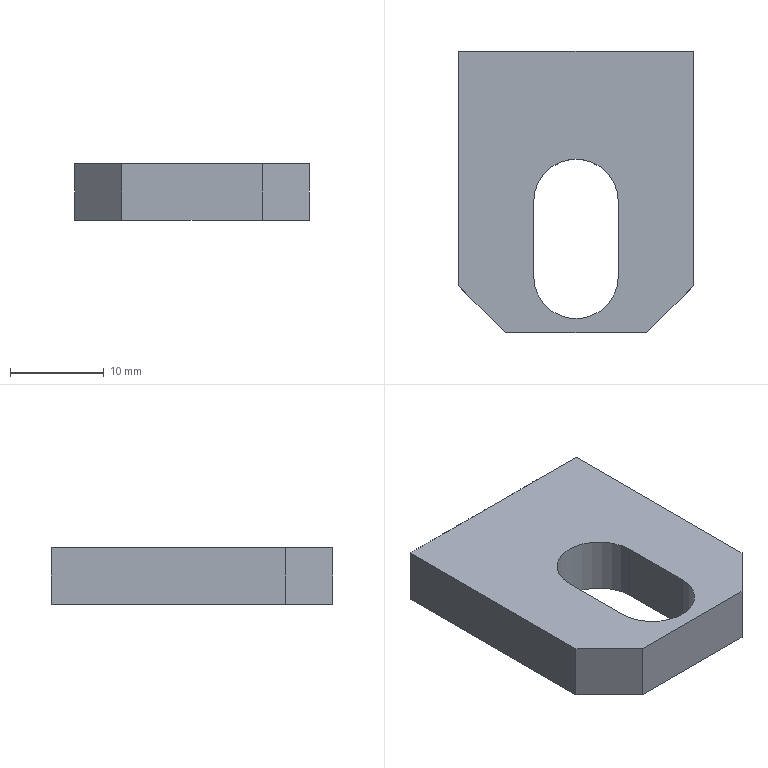Part | NX | features BREP 1 | 1 solid | 16 faces | box 25 x 30 x 6 mm | volume 3358 mm3 | plane 10 | cylinder 4 | cone 2 | commonest cylinder face diameters 3.3 x2 9 x2
STEP:
#1=CARTESIAN_POINT('',(-12.5,30.,0.));
#2=VERTEX_POINT('',#1);
#3=CARTESIAN_POINT('',(-12.5,5.,0.));
#4=VERTEX_POINT('',#3);
#5=CARTESIAN_POINT('',(-12.5,30.,0.));
#6=DIRECTION('',(0.,-1.,0.));
#7=VECTOR('',#6,1000.);
#8=LINE('',#5,#7);
#9=EDGE_CURVE('',#2,#4,#8,.T.);
#10=ORIENTED_EDGE('',*,*,#9,.T.);
#11=CARTESIAN_POINT('',(-12.5,5.,6.));
#12=VERTEX_POINT('',#11);
#13=CARTESIAN_POINT('',(-12.5,5.,6.));
#14=DIRECTION('',(0.,0.,1.));
#15=VECTOR('',#14,1000.);
#16=LINE('',#13,#15);
#17=EDGE_CURVE('',#4,#12,#16,.T.);
#18=ORIENTED_EDGE('',*,*,#17,.T.);
#19=CARTESIAN_POINT('',(-12.5,30.,6.));
#20=VERTEX_POINT('',#19);
#21=CARTESIAN_POINT('',(-12.5,30.,6.));
#22=DIRECTION('',(0.,-1.,0.));
#23=VECTOR('',#22,1000.);
#24=LINE('',#21,#23);
#25=EDGE_CURVE('',#20,#12,#24,.T.);
#26=ORIENTED_EDGE('',*,*,#25,.F.);
#27=CARTESIAN_POINT('',(-12.5,30.,6.));
#28=DIRECTION('',(0.,0.,-1.));
#29=VECTOR('',#28,1000.);
#30=LINE('',#27,#29);
#31=EDGE_CURVE('',#20,#2,#30,.T.);
#32=ORIENTED_EDGE('',*,*,#31,.T.);
#33=EDGE_LOOP('',(#10,#18,#26,#32));
#34=FACE_BOUND('',#33,.T.);
#35=CARTESIAN_POINT('',(-12.5,30.,6.));
#36=DIRECTION('',(1.,0.,0.));
#37=DIRECTION('',(0.,-1.,0.));
#38=AXIS2_PLACEMENT_3D('',#35,#36,#37);
#39=PLANE('',#38);
#40=ADVANCED_FACE('',(#34),#39,.F.);
#41=CARTESIAN_POINT('',(-7.5,0.,0.));
#42=VERTEX_POINT('',#41);
#43=CARTESIAN_POINT('',(7.5,0.,0.));
#44=VERTEX_POINT('',#43);
#45=CARTESIAN_POINT('',(-12.5,0.,0.));
#46=DIRECTION('',(1.,0.,0.));
#47=VECTOR('',#46,1000.);
#48=LINE('',#45,#47);
#49=EDGE_CURVE('',#42,#44,#48,.T.);
#50=ORIENTED_EDGE('',*,*,#49,.T.);
#51=CARTESIAN_POINT('',(7.5,0.,6.));
#52=VERTEX_POINT('',#51);
#53=CARTESIAN_POINT('',(7.5,0.,6.));
#54=DIRECTION('',(0.,0.,1.));
#55=VECTOR('',#54,1000.);
#56=LINE('',#53,#55);
#57=EDGE_CURVE('',#44,#52,#56,.T.);
#58=ORIENTED_EDGE('',*,*,#57,.T.);
#59=CARTESIAN_POINT('',(-7.5,0.,6.));
#60=VERTEX_POINT('',#59);
#61=CARTESIAN_POINT('',(-12.5,0.,6.));
#62=DIRECTION('',(1.,0.,0.));
#63=VECTOR('',#62,1000.);
#64=LINE('',#61,#63);
#65=EDGE_CURVE('',#60,#52,#64,.T.);
#66=ORIENTED_EDGE('',*,*,#65,.F.);
#67=CARTESIAN_POINT('',(-7.5,0.,6.));
#68=DIRECTION('',(0.,0.,-1.));
#69=VECTOR('',#68,1000.);
#70=LINE('',#67,#69);
#71=EDGE_CURVE('',#60,#42,#70,.T.);
#72=ORIENTED_EDGE('',*,*,#71,.T.);
#73=EDGE_LOOP('',(#50,#58,#66,#72));
#74=FACE_BOUND('',#73,.T.);
#75=CARTESIAN_POINT('',(-12.5,0.,6.));
#76=DIRECTION('',(0.,1.,0.));
#77=DIRECTION('',(1.,0.,0.));
#78=AXIS2_PLACEMENT_3D('',#75,#76,#77);
#79=PLANE('',#78);
#80=ADVANCED_FACE('',(#74),#79,.F.);
#81=CARTESIAN_POINT('',(12.5,5.,6.));
#82=VERTEX_POINT('',#81);
#83=CARTESIAN_POINT('',(12.5,30.,6.));
#84=VERTEX_POINT('',#83);
#85=CARTESIAN_POINT('',(12.5,0.,6.));
#86=DIRECTION('',(0.,1.,0.));
#87=VECTOR('',#86,1000.);
#88=LINE('',#85,#87);
#89=EDGE_CURVE('',#82,#84,#88,.T.);
#90=ORIENTED_EDGE('',*,*,#89,.F.);
#91=CARTESIAN_POINT('',(12.5,5.,0.));
#92=VERTEX_POINT('',#91);
#93=CARTESIAN_POINT('',(12.5,5.,6.));
#94=DIRECTION('',(0.,0.,-1.));
#95=VECTOR('',#94,1000.);
#96=LINE('',#93,#95);
#97=EDGE_CURVE('',#82,#92,#96,.T.);
#98=ORIENTED_EDGE('',*,*,#97,.T.);
#99=CARTESIAN_POINT('',(12.5,30.,0.));
#100=VERTEX_POINT('',#99);
#101=CARTESIAN_POINT('',(12.5,0.,0.));
#102=DIRECTION('',(0.,1.,0.));
#103=VECTOR('',#102,1000.);
#104=LINE('',#101,#103);
#105=EDGE_CURVE('',#92,#100,#104,.T.);
#106=ORIENTED_EDGE('',*,*,#105,.T.);
#107=CARTESIAN_POINT('',(12.5,30.,6.));
#108=DIRECTION('',(0.,0.,-1.));
#109=VECTOR('',#108,1000.);
#110=LINE('',#107,#109);
#111=EDGE_CURVE('',#84,#100,#110,.T.);
#112=ORIENTED_EDGE('',*,*,#111,.F.);
#113=EDGE_LOOP('',(#90,#98,#106,#112));
#114=FACE_BOUND('',#113,.T.);
#115=CARTESIAN_POINT('',(12.5,0.,6.));
#116=DIRECTION('',(-1.,0.,0.));
#117=DIRECTION('',(0.,0.,-1.));
#118=AXIS2_PLACEMENT_3D('',#115,#116,#117);
#119=PLANE('',#118);
#120=ADVANCED_FACE('',(#114),#119,.F.);
#121=CARTESIAN_POINT('',(-7.5,30.,4.65));
#122=VERTEX_POINT('',#121);
#123=CARTESIAN_POINT('',(-7.5,30.,3.));
#124=DIRECTION('',(0.,1.,0.));
#125=DIRECTION('',(0.,0.,1.));
#126=AXIS2_PLACEMENT_3D('',#123,#124,#125);
#127=CIRCLE('',#126,1.65);
#128=EDGE_CURVE('',#122,#122,#127,.T.);
#129=ORIENTED_EDGE('',*,*,#128,.F.);
#130=EDGE_LOOP('',(#129));
#131=FACE_BOUND('',#130,.T.);
#132=CARTESIAN_POINT('',(7.5,30.,4.65));
#133=VERTEX_POINT('',#132);
#134=CARTESIAN_POINT('',(7.5,30.,3.));
#135=DIRECTION('',(0.,1.,0.));
#136=DIRECTION('',(0.,0.,1.));
#137=AXIS2_PLACEMENT_3D('',#134,#135,#136);
#138=CIRCLE('',#137,1.65);
#139=EDGE_CURVE('',#133,#133,#138,.T.);
#140=ORIENTED_EDGE('',*,*,#139,.F.);
#141=EDGE_LOOP('',(#140));
#142=FACE_BOUND('',#141,.T.);
#143=CARTESIAN_POINT('',(12.5,30.,0.));
#144=DIRECTION('',(-1.,0.,0.));
#145=VECTOR('',#144,1000.);
#146=LINE('',#143,#145);
#147=EDGE_CURVE('',#100,#2,#146,.T.);
#148=ORIENTED_EDGE('',*,*,#147,.T.);
#149=ORIENTED_EDGE('',*,*,#31,.F.);
#150=CARTESIAN_POINT('',(12.5,30.,6.));
#151=DIRECTION('',(-1.,0.,0.));
#152=VECTOR('',#151,1000.);
#153=LINE('',#150,#152);
#154=EDGE_CURVE('',#84,#20,#153,.T.);
#155=ORIENTED_EDGE('',*,*,#154,.F.);
#156=ORIENTED_EDGE('',*,*,#111,.T.);
#157=EDGE_LOOP('',(#148,#149,#155,#156));
#158=FACE_BOUND('',#157,.T.);
#159=CARTESIAN_POINT('',(12.5,30.,6.));
#160=DIRECTION('',(0.,-1.,0.));
#161=DIRECTION('',(-1.,0.,0.));
#162=AXIS2_PLACEMENT_3D('',#159,#160,#161);
#163=PLANE('',#162);
#164=ADVANCED_FACE('',(#131,#142,#158),#163,.F.);
#165=CARTESIAN_POINT('',(-4.5,6.,6.));
#166=VERTEX_POINT('',#165);
#167=CARTESIAN_POINT('',(4.5,6.,6.));
#168=VERTEX_POINT('',#167);
#169=CARTESIAN_POINT('',(0.,6.,6.));
#170=DIRECTION('',(0.,0.,1.));
#171=DIRECTION('',(1.,0.,0.));
#172=AXIS2_PLACEMENT_3D('',#169,#170,#171);
#173=CIRCLE('',#172,4.5);
#174=EDGE_CURVE('',#166,#168,#173,.T.);
#175=ORIENTED_EDGE('',*,*,#174,.F.);
#176=CARTESIAN_POINT('',(-4.5,14.,6.));
#177=VERTEX_POINT('',#176);
#178=CARTESIAN_POINT('',(-4.5,0.,6.));
#179=DIRECTION('',(0.,-1.,0.));
#180=VECTOR('',#179,1000.);
#181=LINE('',#178,#180);
#182=EDGE_CURVE('',#177,#166,#181,.T.);
#183=ORIENTED_EDGE('',*,*,#182,.F.);
#184=CARTESIAN_POINT('',(4.5,14.,6.));
#185=VERTEX_POINT('',#184);
#186=CARTESIAN_POINT('',(0.,14.,6.));
#187=DIRECTION('',(0.,0.,1.));
#188=DIRECTION('',(1.,0.,0.));
#189=AXIS2_PLACEMENT_3D('',#186,#187,#188);
#190=CIRCLE('',#189,4.5);
#191=EDGE_CURVE('',#185,#177,#190,.T.);
#192=ORIENTED_EDGE('',*,*,#191,.F.);
#193=CARTESIAN_POINT('',(4.5,0.,6.));
#194=DIRECTION('',(0.,1.,0.));
#195=VECTOR('',#194,1000.);
#196=LINE('',#193,#195);
#197=EDGE_CURVE('',#168,#185,#196,.T.);
#198=ORIENTED_EDGE('',*,*,#197,.F.);
#199=EDGE_LOOP('',(#175,#183,#192,#198));
#200=FACE_BOUND('',#199,.T.);
#201=ORIENTED_EDGE('',*,*,#65,.T.);
#202=CARTESIAN_POINT('',(3.75,-3.75,6.));
#203=DIRECTION('',(0.7071,0.7071,0.));
#204=VECTOR('',#203,1000.);
#205=LINE('',#202,#204);
#206=EDGE_CURVE('',#52,#82,#205,.T.);
#207=ORIENTED_EDGE('',*,*,#206,.T.);
#208=ORIENTED_EDGE('',*,*,#89,.T.);
#209=ORIENTED_EDGE('',*,*,#154,.T.);
#210=ORIENTED_EDGE('',*,*,#25,.T.);
#211=CARTESIAN_POINT('',(-3.75,-3.75,6.));
#212=DIRECTION('',(0.7071,-0.7071,0.));
#213=VECTOR('',#212,1000.);
#214=LINE('',#211,#213);
#215=EDGE_CURVE('',#12,#60,#214,.T.);
#216=ORIENTED_EDGE('',*,*,#215,.T.);
#217=EDGE_LOOP('',(#201,#207,#208,#209,#210,#216));
#218=FACE_BOUND('',#217,.T.);
#219=CARTESIAN_POINT('',(0.,0.,6.));
#220=DIRECTION('',(0.,0.,1.));
#221=DIRECTION('',(-1.,0.,0.));
#222=AXIS2_PLACEMENT_3D('',#219,#220,#221);
#223=PLANE('',#222);
#224=ADVANCED_FACE('',(#200,#218),#223,.T.);
#225=CARTESIAN_POINT('',(-4.5,6.,0.));
#226=VERTEX_POINT('',#225);
#227=CARTESIAN_POINT('',(-4.5,14.,0.));
#228=VERTEX_POINT('',#227);
#229=CARTESIAN_POINT('',(-4.5,6.,0.));
#230=DIRECTION('',(0.,1.,0.));
#231=VECTOR('',#230,1000.);
#232=LINE('',#229,#231);
#233=EDGE_CURVE('',#226,#228,#232,.T.);
#234=ORIENTED_EDGE('',*,*,#233,.F.);
#235=CARTESIAN_POINT('',(4.5,6.,0.));
#236=VERTEX_POINT('',#235);
#237=CARTESIAN_POINT('',(0.,6.,0.));
#238=DIRECTION('',(0.,0.,-1.));
#239=DIRECTION('',(-1.,0.,0.));
#240=AXIS2_PLACEMENT_3D('',#237,#238,#239);
#241=CIRCLE('',#240,4.5);
#242=EDGE_CURVE('',#236,#226,#241,.T.);
#243=ORIENTED_EDGE('',*,*,#242,.F.);
#244=CARTESIAN_POINT('',(4.5,14.,0.));
#245=VERTEX_POINT('',#244);
#246=CARTESIAN_POINT('',(4.5,6.,0.));
#247=DIRECTION('',(0.,-1.,0.));
#248=VECTOR('',#247,1000.);
#249=LINE('',#246,#248);
#250=EDGE_CURVE('',#245,#236,#249,.T.);
#251=ORIENTED_EDGE('',*,*,#250,.F.);
#252=CARTESIAN_POINT('',(0.,14.,0.));
#253=DIRECTION('',(0.,0.,-1.));
#254=DIRECTION('',(-1.,0.,0.));
#255=AXIS2_PLACEMENT_3D('',#252,#253,#254);
#256=CIRCLE('',#255,4.5);
#257=EDGE_CURVE('',#228,#245,#256,.T.);
#258=ORIENTED_EDGE('',*,*,#257,.F.);
#259=EDGE_LOOP('',(#234,#243,#251,#258));
#260=FACE_BOUND('',#259,.T.);
#261=ORIENTED_EDGE('',*,*,#105,.F.);
#262=CARTESIAN_POINT('',(12.5,5.,0.));
#263=DIRECTION('',(-0.7071,-0.7071,0.));
#264=VECTOR('',#263,1000.);
#265=LINE('',#262,#264);
#266=EDGE_CURVE('',#92,#44,#265,.T.);
#267=ORIENTED_EDGE('',*,*,#266,.T.);
#268=ORIENTED_EDGE('',*,*,#49,.F.);
#269=CARTESIAN_POINT('',(-7.5,0.,0.));
#270=DIRECTION('',(-0.7071,0.7071,0.));
#271=VECTOR('',#270,1000.);
#272=LINE('',#269,#271);
#273=EDGE_CURVE('',#42,#4,#272,.T.);
#274=ORIENTED_EDGE('',*,*,#273,.T.);
#275=ORIENTED_EDGE('',*,*,#9,.F.);
#276=ORIENTED_EDGE('',*,*,#147,.F.);
#277=EDGE_LOOP('',(#261,#267,#268,#274,#275,#276));
#278=FACE_BOUND('',#277,.T.);
#279=CARTESIAN_POINT('',(0.,0.,0.));
#280=DIRECTION('',(0.,0.,1.));
#281=DIRECTION('',(-1.,0.,0.));
#282=AXIS2_PLACEMENT_3D('',#279,#280,#281);
#283=PLANE('',#282);
#284=ADVANCED_FACE('',(#260,#278),#283,.F.);
#285=ORIENTED_EDGE('',*,*,#174,.T.);
#286=CARTESIAN_POINT('',(4.5,6.,16.));
#287=DIRECTION('',(0.,0.,-1.));
#288=VECTOR('',#287,1000.);
#289=LINE('',#286,#288);
#290=EDGE_CURVE('',#168,#236,#289,.T.);
#291=ORIENTED_EDGE('',*,*,#290,.T.);
#292=ORIENTED_EDGE('',*,*,#242,.T.);
#293=CARTESIAN_POINT('',(-4.5,6.,16.));
#294=DIRECTION('',(0.,0.,-1.));
#295=VECTOR('',#294,1000.);
#296=LINE('',#293,#295);
#297=EDGE_CURVE('',#166,#226,#296,.T.);
#298=ORIENTED_EDGE('',*,*,#297,.F.);
#299=EDGE_LOOP('',(#285,#291,#292,#298));
#300=FACE_BOUND('',#299,.T.);
#301=CARTESIAN_POINT('',(0.,6.,16.));
#302=DIRECTION('',(0.,0.,-1.));
#303=DIRECTION('',(1.,0.,0.));
#304=AXIS2_PLACEMENT_3D('',#301,#302,#303);
#305=CYLINDRICAL_SURFACE('',#304,4.5);
#306=ADVANCED_FACE('',(#300),#305,.F.);
#307=ORIENTED_EDGE('',*,*,#197,.T.);
#308=CARTESIAN_POINT('',(4.5,14.,16.));
#309=DIRECTION('',(0.,0.,-1.));
#310=VECTOR('',#309,1000.);
#311=LINE('',#308,#310);
#312=EDGE_CURVE('',#185,#245,#311,.T.);
#313=ORIENTED_EDGE('',*,*,#312,.T.);
#314=ORIENTED_EDGE('',*,*,#250,.T.);
#315=ORIENTED_EDGE('',*,*,#290,.F.);
#316=EDGE_LOOP('',(#307,#313,#314,#315));
#317=FACE_BOUND('',#316,.T.);
#318=CARTESIAN_POINT('',(4.5,6.,16.));
#319=DIRECTION('',(1.,0.,0.));
#320=DIRECTION('',(0.,-1.,0.));
#321=AXIS2_PLACEMENT_3D('',#318,#319,#320);
#322=PLANE('',#321);
#323=ADVANCED_FACE('',(#317),#322,.F.);
#324=ORIENTED_EDGE('',*,*,#191,.T.);
#325=CARTESIAN_POINT('',(-4.5,14.,16.));
#326=DIRECTION('',(0.,0.,-1.));
#327=VECTOR('',#326,1000.);
#328=LINE('',#325,#327);
#329=EDGE_CURVE('',#177,#228,#328,.T.);
#330=ORIENTED_EDGE('',*,*,#329,.T.);
#331=ORIENTED_EDGE('',*,*,#257,.T.);
#332=ORIENTED_EDGE('',*,*,#312,.F.);
#333=EDGE_LOOP('',(#324,#330,#331,#332));
#334=FACE_BOUND('',#333,.T.);
#335=CARTESIAN_POINT('',(0.,14.,16.));
#336=DIRECTION('',(0.,0.,-1.));
#337=DIRECTION('',(1.,0.,0.));
#338=AXIS2_PLACEMENT_3D('',#335,#336,#337);
#339=CYLINDRICAL_SURFACE('',#338,4.5);
#340=ADVANCED_FACE('',(#334),#339,.F.);
#341=ORIENTED_EDGE('',*,*,#182,.T.);
#342=ORIENTED_EDGE('',*,*,#297,.T.);
#343=ORIENTED_EDGE('',*,*,#233,.T.);
#344=ORIENTED_EDGE('',*,*,#329,.F.);
#345=EDGE_LOOP('',(#341,#342,#343,#344));
#346=FACE_BOUND('',#345,.T.);
#347=CARTESIAN_POINT('',(-4.5,6.,16.));
#348=DIRECTION('',(-1.,0.,0.));
#349=DIRECTION('',(0.,1.,0.));
#350=AXIS2_PLACEMENT_3D('',#347,#348,#349);
#351=PLANE('',#350);
#352=ADVANCED_FACE('',(#346),#351,.F.);
#353=ORIENTED_EDGE('',*,*,#206,.F.);
#354=ORIENTED_EDGE('',*,*,#57,.F.);
#355=ORIENTED_EDGE('',*,*,#266,.F.);
#356=ORIENTED_EDGE('',*,*,#97,.F.);
#357=EDGE_LOOP('',(#353,#354,#355,#356));
#358=FACE_BOUND('',#357,.T.);
#359=CARTESIAN_POINT('',(12.5,5.,6.));
#360=DIRECTION('',(-0.7071,0.7071,0.));
#361=DIRECTION('',(0.,0.,1.));
#362=AXIS2_PLACEMENT_3D('',#359,#360,#361);
#363=PLANE('',#362);
#364=ADVANCED_FACE('',(#358),#363,.F.);
#365=ORIENTED_EDGE('',*,*,#215,.F.);
#366=ORIENTED_EDGE('',*,*,#17,.F.);
#367=ORIENTED_EDGE('',*,*,#273,.F.);
#368=ORIENTED_EDGE('',*,*,#71,.F.);
#369=EDGE_LOOP('',(#365,#366,#367,#368));
#370=FACE_BOUND('',#369,.T.);
#371=CARTESIAN_POINT('',(-7.5,0.,6.));
#372=DIRECTION('',(0.7071,0.7071,0.));
#373=DIRECTION('',(0.,0.,1.));
#374=AXIS2_PLACEMENT_3D('',#371,#372,#373);
#375=PLANE('',#374);
#376=ADVANCED_FACE('',(#370),#375,.F.);
#377=CARTESIAN_POINT('',(7.5,18.909,3.));
#378=VERTEX_POINT('',#377);
#379=VERTEX_LOOP('',#378);
#380=FACE_BOUND('',#379,.T.);
#381=CARTESIAN_POINT('',(7.5,19.9,4.65));
#382=VERTEX_POINT('',#381);
#383=CARTESIAN_POINT('',(7.5,19.9,3.));
#384=DIRECTION('',(0.,1.,0.));
#385=DIRECTION('',(0.,0.,1.));
#386=AXIS2_PLACEMENT_3D('',#383,#384,#385);
#387=CIRCLE('',#386,1.65);
#388=EDGE_CURVE('',#382,#382,#387,.T.);
#389=ORIENTED_EDGE('',*,*,#388,.T.);
#390=EDGE_LOOP('',(#389));
#391=FACE_BOUND('',#390,.T.);
#392=CARTESIAN_POINT('',(7.5,19.9,3.));
#393=DIRECTION('',(0.,1.,0.));
#394=DIRECTION('',(0.,0.,-1.));
#395=AXIS2_PLACEMENT_3D('',#392,#393,#394);
#396=CONICAL_SURFACE('',#395,1.65,1.03);
#397=ADVANCED_FACE('',(#380,#391),#396,.F.);
#398=ORIENTED_EDGE('',*,*,#388,.F.);
#399=EDGE_LOOP('',(#398));
#400=FACE_BOUND('',#399,.T.);
#401=ORIENTED_EDGE('',*,*,#139,.T.);
#402=EDGE_LOOP('',(#401));
#403=FACE_BOUND('',#402,.T.);
#404=CARTESIAN_POINT('',(7.5,30.,3.));
#405=DIRECTION('',(0.,1.,0.));
#406=DIRECTION('',(0.,0.,-1.));
#407=AXIS2_PLACEMENT_3D('',#404,#405,#406);
#408=CYLINDRICAL_SURFACE('',#407,1.65);
#409=ADVANCED_FACE('',(#400,#403),#408,.F.);
#410=CARTESIAN_POINT('',(-7.5,18.909,3.));
#411=VERTEX_POINT('',#410);
#412=VERTEX_LOOP('',#411);
#413=FACE_BOUND('',#412,.T.);
#414=CARTESIAN_POINT('',(-7.5,19.9,4.65));
#415=VERTEX_POINT('',#414);
#416=CARTESIAN_POINT('',(-7.5,19.9,3.));
#417=DIRECTION('',(0.,1.,0.));
#418=DIRECTION('',(0.,0.,1.));
#419=AXIS2_PLACEMENT_3D('',#416,#417,#418);
#420=CIRCLE('',#419,1.65);
#421=EDGE_CURVE('',#415,#415,#420,.T.);
#422=ORIENTED_EDGE('',*,*,#421,.T.);
#423=EDGE_LOOP('',(#422));
#424=FACE_BOUND('',#423,.T.);
#425=CARTESIAN_POINT('',(-7.5,19.9,3.));
#426=DIRECTION('',(0.,1.,0.));
#427=DIRECTION('',(0.,0.,-1.));
#428=AXIS2_PLACEMENT_3D('',#425,#426,#427);
#429=CONICAL_SURFACE('',#428,1.65,1.03);
#430=ADVANCED_FACE('',(#413,#424),#429,.F.);
#431=ORIENTED_EDGE('',*,*,#421,.F.);
#432=EDGE_LOOP('',(#431));
#433=FACE_BOUND('',#432,.T.);
#434=ORIENTED_EDGE('',*,*,#128,.T.);
#435=EDGE_LOOP('',(#434));
#436=FACE_BOUND('',#435,.T.);
#437=CARTESIAN_POINT('',(-7.5,30.,3.));
#438=DIRECTION('',(0.,1.,0.));
#439=DIRECTION('',(0.,0.,-1.));
#440=AXIS2_PLACEMENT_3D('',#437,#438,#439);
#441=CYLINDRICAL_SURFACE('',#440,1.65);
#442=ADVANCED_FACE('',(#433,#436),#441,.F.);
#443=CLOSED_SHELL('',(#40,#80,#120,#164,#224,#284,#306,#323,#340,#352,#364,#376,#397,#409,#430,#442));
#444=MANIFOLD_SOLID_BREP('',#443);
#445=(LENGTH_UNIT()NAMED_UNIT(*)SI_UNIT(.MILLI.,.METRE.));
#446=UNCERTAINTY_MEASURE_WITH_UNIT(LENGTH_MEASURE(0.00001),#445,'','');
#447=(NAMED_UNIT(*)PLANE_ANGLE_UNIT()SI_UNIT($,.RADIAN.));
#448=(NAMED_UNIT(*)SI_UNIT($,.STERADIAN.)SOLID_ANGLE_UNIT());
#449=(GEOMETRIC_REPRESENTATION_CONTEXT(3)GLOBAL_UNCERTAINTY_ASSIGNED_CONTEXT((#446))GLOBAL_UNIT_ASSIGNED_CONTEXT((#445,#447,#448))REPRESENTATION_CONTEXT('',''));
#450=ADVANCED_BREP_SHAPE_REPRESENTATION('',(#444),#449);